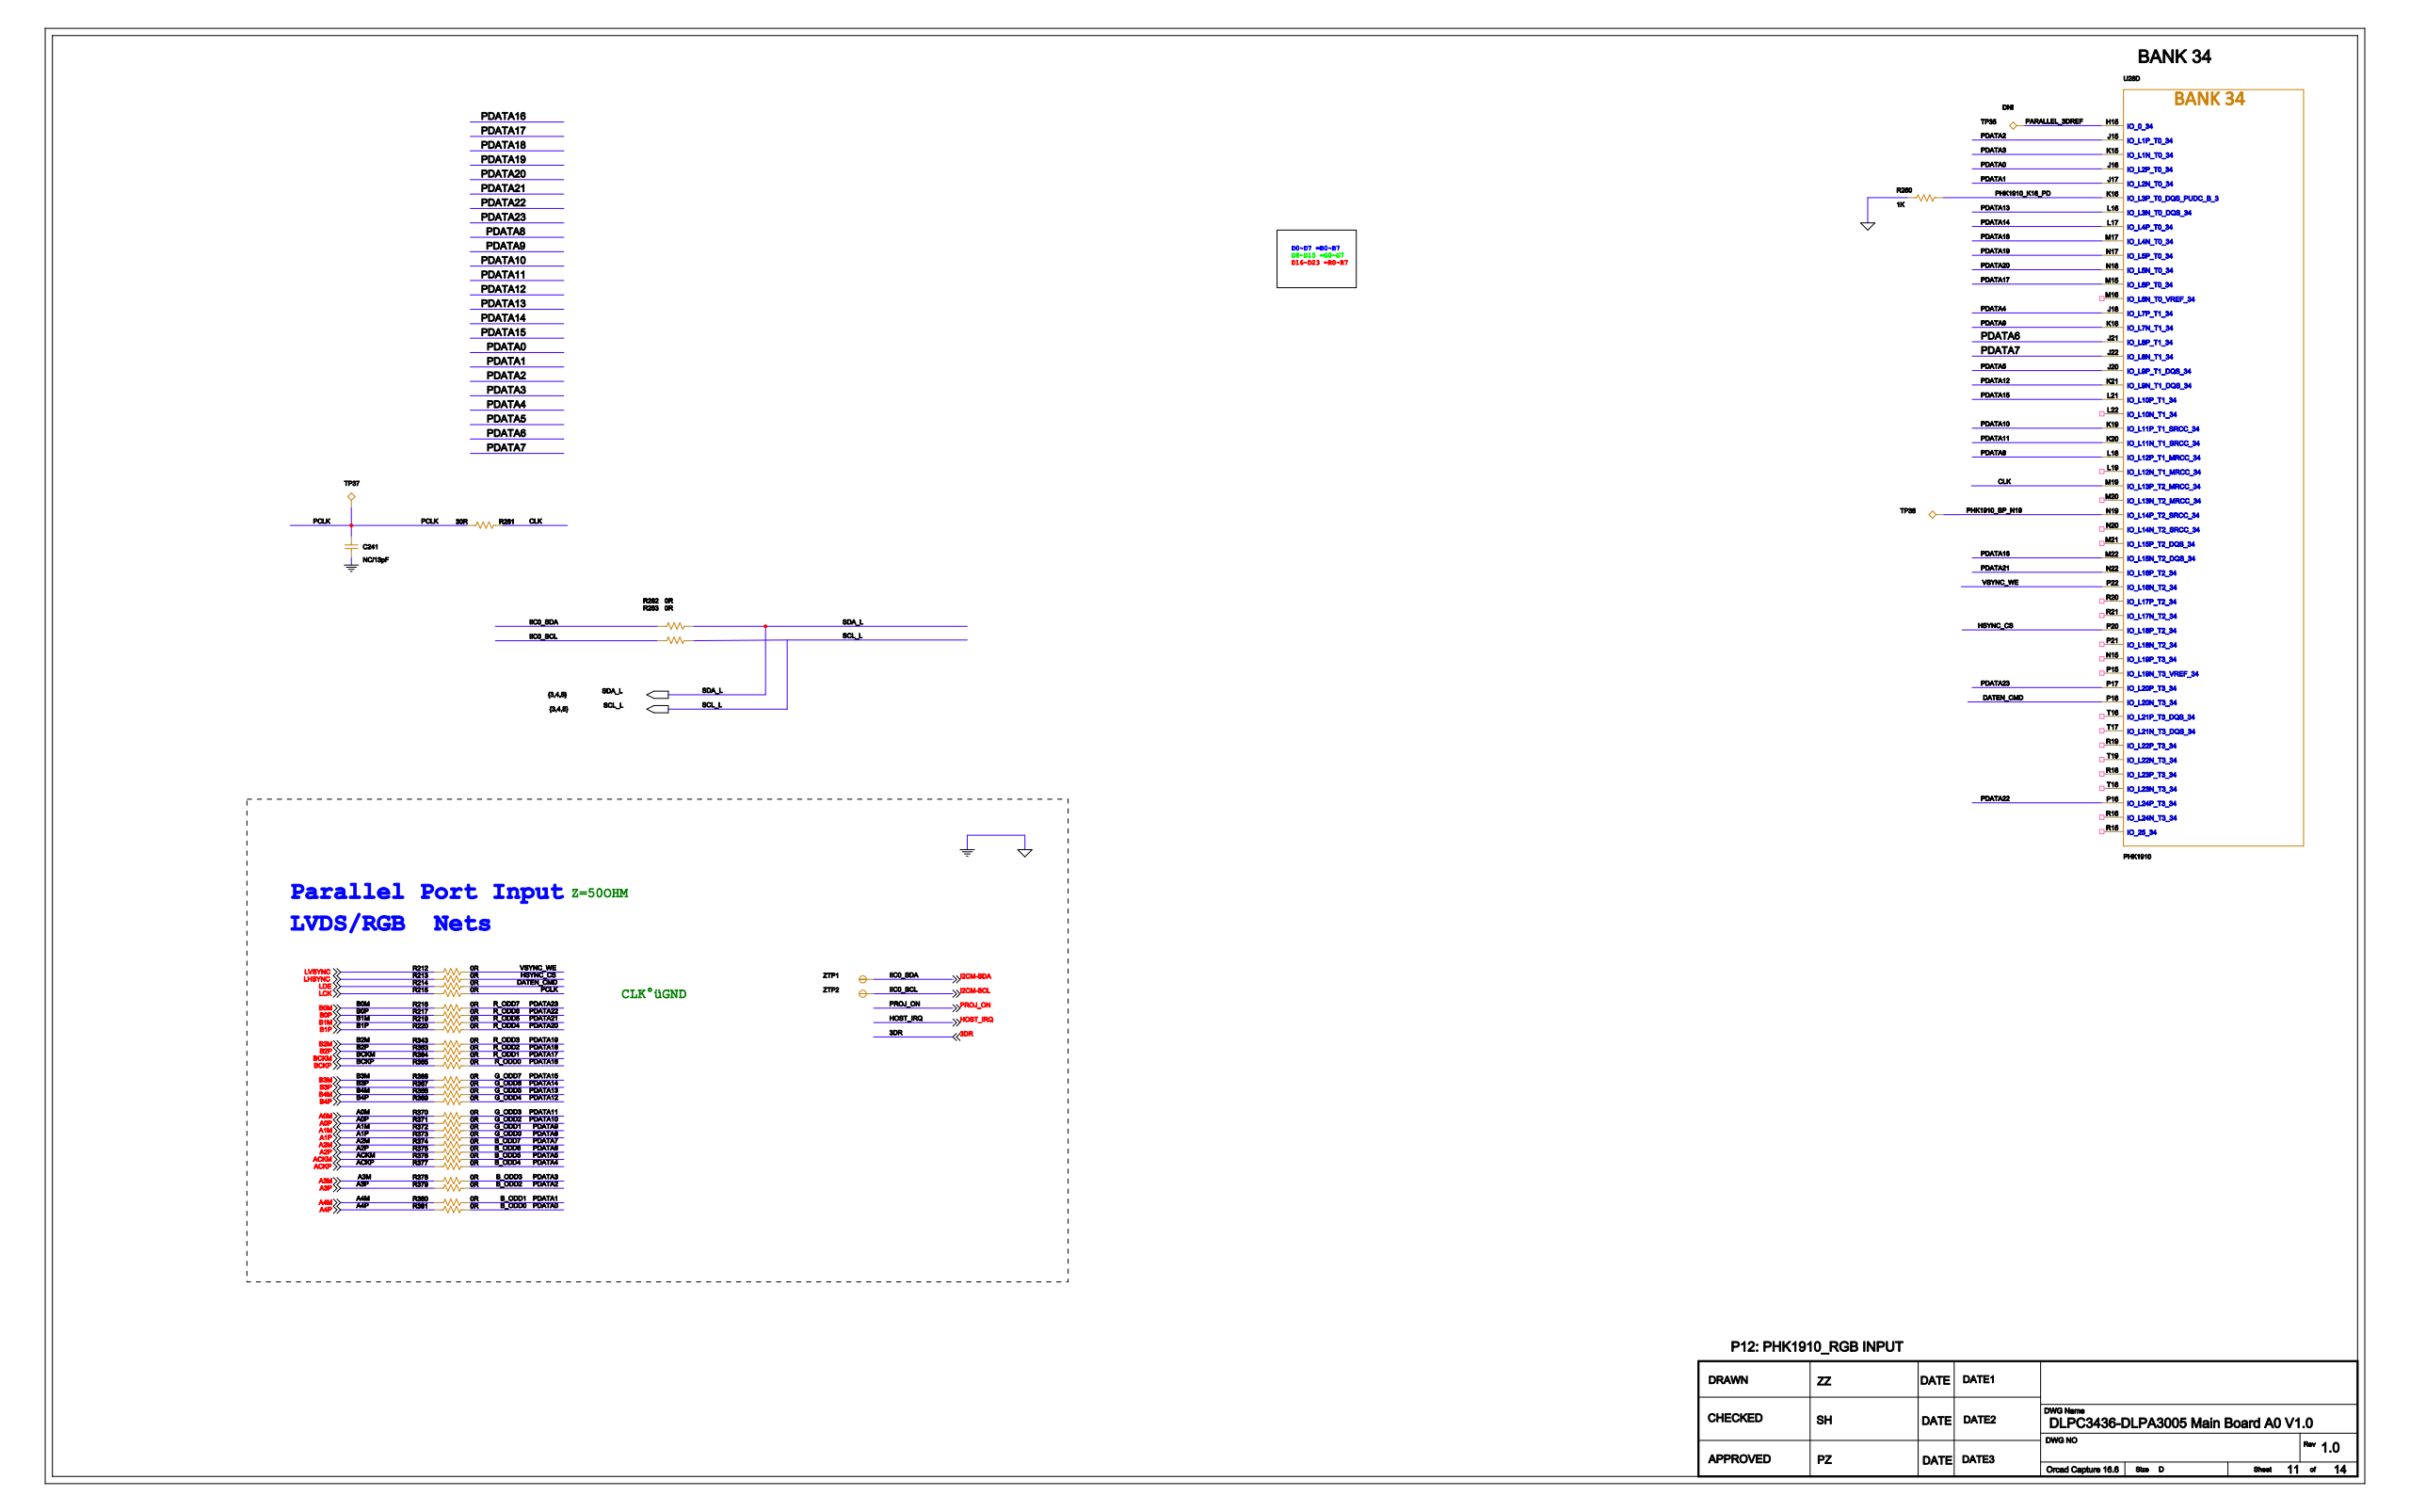Circuit board | Cadence Allegro | 1223 parts | 777 nets | one sheet of the schematic
Parts on this sheet (reference | value | footprint):
C241 | NC/13pF | C0402
R212 | 0R | R0201
R213 | 0R | R0201
R214 | 0R | R0201
R215 | 0R | R0201
R216 | 0R | R0201
R217 | 0R | R0201
R219 | 0R | R0201
R220 | 0R | R0201
R260 | 1K | R0201
R261 | 30R | R0201
R262 | 0R | R0201
R263 | 0R | R0201
R343 | 0R | R0201
R363 | 0R | R0201
R364 | 0R | R0201
R365 | 0R | R0201
R366 | 0R | R0201
R367 | 0R | R0201
R368 | 0R | R0201
R369 | 0R | R0201
R370 | 0R | R0201
R371 | 0R | R0201
R372 | 0R | R0201
R373 | 0R | R0201
R374 | 0R | R0201
R375 | 0R | R0201
R376 | 0R | R0201
R377 | 0R | R0201
R378 | 0R | R0201
R379 | 0R | R0201
R380 | 0R | R0201
R381 | 0R | R0201
TP35 | TP40 | TP06MM
TP36 | TP40 | TP06MM
TP37 | TP40 | TP06MM
U28 | PHK1910 | XILINX_CLG484
ZTP1 | TP_20RD10 | TP06MM
ZTP2 | TP_20RD10 | TP06MM
Nets of these parts (net: part-pin ...):
GND: C241-2 R260-2 U28-P12
PCLK: C241-1 R215-2 R261-1 TP37-1
PARALLEL_3DREF: TP35-1 U28-H15
PHK1910_SP_N19: TP36-1 U28-N19
CLK: R261-2 U28-M19
LVSYNC: R212-1
VSYNC_WE: R212-2 U28-P22
LHSYNC: R213-1
HSYNC_CS: R213-2 U28-P20
LDE: R214-1
DATEN_CMD: R214-2 U28-P18
LCK: R215-1
B0M: R216-1
PDATA23: R216-2 U28-P17
B0P: R217-1
PDATA22: R217-2 U28-P16
B1M: R219-1
PDATA21: R219-2 U28-N22
B1P: R220-1
PDATA20: R220-2 U28-N18
I2CM-SDA: R262-1 ZTP1-1
SDA_L: R262-2
I2CM-SCL: R263-1 ZTP2-1
SCL_L: R263-2
B2M: R343-1
PDATA19: R343-2 U28-N17
B2P: R363-1
PDATA18: R363-2 U28-M17
BCKM: R364-1
PDATA17: R364-2 U28-M15
BCKP: R365-1
PDATA16: R365-2 U28-M22
B3M: R366-1
G_ODD7: R366-2 U28-L21
B3P: R367-1
G_ODD6: R367-2 U28-L17
B4M: R368-1
G_ODD5: R368-2 U28-L16
B4P: R369-1
G_ODD4: R369-2 U28-K21
A0M: R370-1
G_ODD3: R370-2 U28-K20
A0P: R371-1
G_ODD2: R371-2 U28-K19
A1M: R372-1
G_ODD1: R372-2 U28-K18
A1P: R373-1
G_ODD0: R373-2 U28-L18
A2M: R374-1
B_ODD7: R374-2 U28-J22
A2P: R375-1
B_ODD6: R375-2 U28-J21
ACKM: R376-1
B_ODD5: R376-2 U28-J20
ACKP: R377-1
B_ODD4: R377-2 U28-J18
A3M: R378-1
B_ODD3: R378-2 U28-K15
A3P: R379-1
B_ODD2: R379-2 U28-J15
A4M: R380-1
B_ODD1: R380-2 U28-J17
A4P: R381-1
B_ODD0: R381-2 U28-J16
PHK1910_K16_PD: R260-1 U28-K16